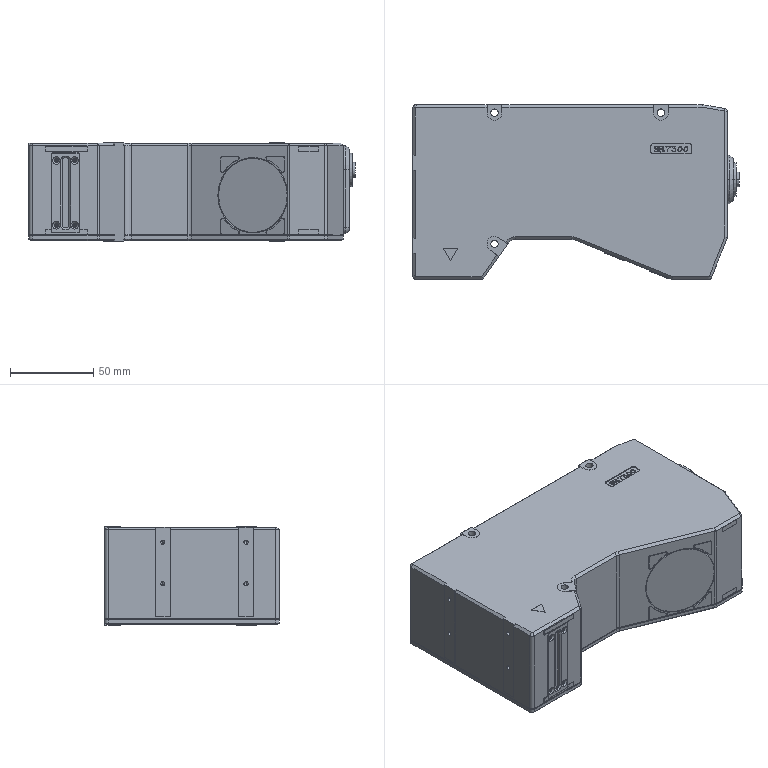Part | SolidWorks | features BaseBody 3 | 2 solids | 740 faces | box 196.4 x 105.4 x 59 mm | volume 1042939 mm3 | plane 382 | cylinder 162 | spline 136 | cone 58 | torus 2 | commonest cylinder face diameters 2 x26 3 x20 4 x16 2.5 x14 1.6 x8 2.542 x8